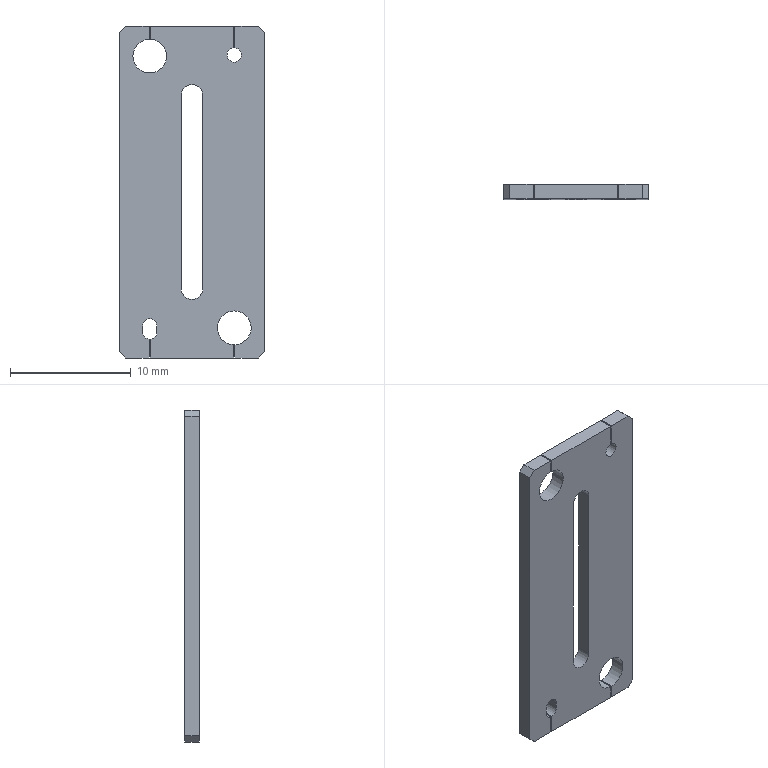Part | SolidWorks | features ICE 3, HoleWzd 2, Chamfer 1, Extrusion 1 | 1 solid | 37 faces | box 12 x 1.2 x 27.5 mm | volume 338.908 mm3 | plane 26 | cylinder 11 | commonest cylinder face diameters 1.2 x5 1.8 x3 2.8 x3
STEP:
#1=CARTESIAN_POINT('',(-3.5,-0.6,-10.5));
#2=VERTEX_POINT('',#1);
#3=CARTESIAN_POINT('',(-2.9,-0.6,-11.1));
#4=VERTEX_POINT('',#3);
#5=CARTESIAN_POINT('',(-3.5,-0.6,-11.1));
#6=DIRECTION('',(0.,1.,0.));
#7=DIRECTION('',(0.,0.,1.));
#8=AXIS2_PLACEMENT_3D('',#5,#6,#7);
#9=CIRCLE('',#8,0.6);
#10=EDGE_CURVE('',#2,#4,#9,.T.);
#11=ORIENTED_EDGE('',*,*,#10,.F.);
#12=CARTESIAN_POINT('',(-3.5,0.6,-10.5));
#13=VERTEX_POINT('',#12);
#14=CARTESIAN_POINT('',(-3.5,-0.6,-10.5));
#15=DIRECTION('',(0.,1.,0.));
#16=VECTOR('',#15,1000.);
#17=LINE('',#14,#16);
#18=EDGE_CURVE('',#2,#13,#17,.T.);
#19=ORIENTED_EDGE('',*,*,#18,.T.);
#20=CARTESIAN_POINT('',(-2.9,0.6,-11.1));
#21=VERTEX_POINT('',#20);
#22=CARTESIAN_POINT('',(-3.5,0.6,-11.1));
#23=DIRECTION('',(0.,1.,0.));
#24=DIRECTION('',(0.,0.,1.));
#25=AXIS2_PLACEMENT_3D('',#22,#23,#24);
#26=CIRCLE('',#25,0.6);
#27=EDGE_CURVE('',#13,#21,#26,.T.);
#28=ORIENTED_EDGE('',*,*,#27,.T.);
#29=CARTESIAN_POINT('',(-2.9,-0.6,-11.1));
#30=DIRECTION('',(0.,1.,0.));
#31=VECTOR('',#30,1000.);
#32=LINE('',#29,#31);
#33=EDGE_CURVE('',#4,#21,#32,.T.);
#34=ORIENTED_EDGE('',*,*,#33,.F.);
#35=EDGE_LOOP('',(#11,#19,#28,#34));
#36=FACE_OUTER_BOUND('',#35,.T.);
#37=CARTESIAN_POINT('',(-3.5,-0.6,-11.1));
#38=DIRECTION('',(0.,1.,0.));
#39=DIRECTION('',(0.,0.,1.));
#40=AXIS2_PLACEMENT_3D('',#37,#38,#39);
#41=CYLINDRICAL_SURFACE('',#40,0.6);
#42=ADVANCED_FACE('',(#36),#41,.F.);
#43=CARTESIAN_POINT('',(3.5,-0.6,-9.85));
#44=VERTEX_POINT('',#43);
#45=CARTESIAN_POINT('',(3.55,-0.6,-12.649));
#46=VERTEX_POINT('',#45);
#47=CARTESIAN_POINT('',(3.5,-0.6,-11.25));
#48=DIRECTION('',(0.,1.,0.));
#49=DIRECTION('',(0.,0.,1.));
#50=AXIS2_PLACEMENT_3D('',#47,#48,#49);
#51=CIRCLE('',#50,1.4);
#52=EDGE_CURVE('',#44,#46,#51,.T.);
#53=ORIENTED_EDGE('',*,*,#52,.F.);
#54=CARTESIAN_POINT('',(3.5,0.6,-9.85));
#55=VERTEX_POINT('',#54);
#56=CARTESIAN_POINT('',(3.5,0.6,-9.85));
#57=DIRECTION('',(0.,1.,0.));
#58=VECTOR('',#57,1000.);
#59=LINE('',#56,#58);
#60=EDGE_CURVE('',#44,#55,#59,.T.);
#61=ORIENTED_EDGE('',*,*,#60,.T.);
#62=CARTESIAN_POINT('',(3.55,0.6,-12.649));
#63=VERTEX_POINT('',#62);
#64=CARTESIAN_POINT('',(3.5,0.6,-11.25));
#65=DIRECTION('',(0.,1.,0.));
#66=DIRECTION('',(0.,0.,1.));
#67=AXIS2_PLACEMENT_3D('',#64,#65,#66);
#68=CIRCLE('',#67,1.4);
#69=EDGE_CURVE('',#55,#63,#68,.T.);
#70=ORIENTED_EDGE('',*,*,#69,.T.);
#71=CARTESIAN_POINT('',(3.55,0.6,-12.649));
#72=DIRECTION('',(0.,-1.,0.));
#73=VECTOR('',#72,1000.);
#74=LINE('',#71,#73);
#75=EDGE_CURVE('',#63,#46,#74,.T.);
#76=ORIENTED_EDGE('',*,*,#75,.T.);
#77=EDGE_LOOP('',(#53,#61,#70,#76));
#78=FACE_OUTER_BOUND('',#77,.T.);
#79=CARTESIAN_POINT('',(3.5,0.6,-11.25));
#80=DIRECTION('',(0.,1.,0.));
#81=DIRECTION('',(0.,0.,1.));
#82=AXIS2_PLACEMENT_3D('',#79,#80,#81);
#83=CYLINDRICAL_SURFACE('',#82,1.4);
#84=ADVANCED_FACE('',(#78),#83,.F.);
#85=CARTESIAN_POINT('',(0.,-0.6,8.9));
#86=VERTEX_POINT('',#85);
#87=CARTESIAN_POINT('',(0.9,-0.6,8.));
#88=VERTEX_POINT('',#87);
#89=CARTESIAN_POINT('',(0.,-0.6,8.));
#90=DIRECTION('',(0.,1.,0.));
#91=DIRECTION('',(0.,0.,1.));
#92=AXIS2_PLACEMENT_3D('',#89,#90,#91);
#93=CIRCLE('',#92,0.9);
#94=EDGE_CURVE('',#86,#88,#93,.T.);
#95=ORIENTED_EDGE('',*,*,#94,.F.);
#96=CARTESIAN_POINT('',(0.,0.6,8.9));
#97=VERTEX_POINT('',#96);
#98=CARTESIAN_POINT('',(0.,-0.6,8.9));
#99=DIRECTION('',(0.,1.,0.));
#100=VECTOR('',#99,1000.);
#101=LINE('',#98,#100);
#102=EDGE_CURVE('',#86,#97,#101,.T.);
#103=ORIENTED_EDGE('',*,*,#102,.T.);
#104=CARTESIAN_POINT('',(0.9,0.6,8.));
#105=VERTEX_POINT('',#104);
#106=CARTESIAN_POINT('',(0.,0.6,8.));
#107=DIRECTION('',(0.,1.,0.));
#108=DIRECTION('',(0.,0.,1.));
#109=AXIS2_PLACEMENT_3D('',#106,#107,#108);
#110=CIRCLE('',#109,0.9);
#111=EDGE_CURVE('',#97,#105,#110,.T.);
#112=ORIENTED_EDGE('',*,*,#111,.T.);
#113=CARTESIAN_POINT('',(0.9,-0.6,8.));
#114=DIRECTION('',(0.,1.,0.));
#115=VECTOR('',#114,1000.);
#116=LINE('',#113,#115);
#117=EDGE_CURVE('',#88,#105,#116,.T.);
#118=ORIENTED_EDGE('',*,*,#117,.F.);
#119=EDGE_LOOP('',(#95,#103,#112,#118));
#120=FACE_OUTER_BOUND('',#119,.T.);
#121=CARTESIAN_POINT('',(0.,-0.6,8.));
#122=DIRECTION('',(0.,1.,0.));
#123=DIRECTION('',(0.,0.,1.));
#124=AXIS2_PLACEMENT_3D('',#121,#122,#123);
#125=CYLINDRICAL_SURFACE('',#124,0.9);
#126=ADVANCED_FACE('',(#120),#125,.F.);
#127=CARTESIAN_POINT('',(3.45,-0.6,-13.75));
#128=VERTEX_POINT('',#127);
#129=CARTESIAN_POINT('',(-3.45,-0.6,-13.75));
#130=VERTEX_POINT('',#129);
#131=CARTESIAN_POINT('',(-6.,-0.6,-13.75));
#132=DIRECTION('',(-1.,0.,0.));
#133=VECTOR('',#132,1000.);
#134=LINE('',#131,#133);
#135=EDGE_CURVE('',#128,#130,#134,.T.);
#136=ORIENTED_EDGE('',*,*,#135,.T.);
#137=CARTESIAN_POINT('',(-3.45,0.6,-13.75));
#138=VERTEX_POINT('',#137);
#139=CARTESIAN_POINT('',(-3.45,-0.6,-13.75));
#140=DIRECTION('',(0.,1.,0.));
#141=VECTOR('',#140,1000.);
#142=LINE('',#139,#141);
#143=EDGE_CURVE('',#130,#138,#142,.T.);
#144=ORIENTED_EDGE('',*,*,#143,.T.);
#145=CARTESIAN_POINT('',(3.45,0.6,-13.75));
#146=VERTEX_POINT('',#145);
#147=CARTESIAN_POINT('',(-6.,0.6,-13.75));
#148=DIRECTION('',(-1.,0.,0.));
#149=VECTOR('',#148,1000.);
#150=LINE('',#147,#149);
#151=EDGE_CURVE('',#146,#138,#150,.T.);
#152=ORIENTED_EDGE('',*,*,#151,.F.);
#153=CARTESIAN_POINT('',(3.45,0.6,-13.75));
#154=DIRECTION('',(0.,-1.,0.));
#155=VECTOR('',#154,1000.);
#156=LINE('',#153,#155);
#157=EDGE_CURVE('',#146,#128,#156,.T.);
#158=ORIENTED_EDGE('',*,*,#157,.T.);
#159=EDGE_LOOP('',(#136,#144,#152,#158));
#160=FACE_OUTER_BOUND('',#159,.T.);
#161=CARTESIAN_POINT('',(-6.,0.6,-13.75));
#162=DIRECTION('',(0.,0.,1.));
#163=DIRECTION('',(1.,0.,0.));
#164=AXIS2_PLACEMENT_3D('',#161,#162,#163);
#165=PLANE('',#164);
#166=ADVANCED_FACE('',(#160),#165,.F.);
#167=CARTESIAN_POINT('',(-2.9,0.6,-11.6));
#168=VERTEX_POINT('',#167);
#169=CARTESIAN_POINT('',(-3.45,0.6,-12.198));
#170=VERTEX_POINT('',#169);
#171=CARTESIAN_POINT('',(-3.5,0.6,-11.6));
#172=DIRECTION('',(0.,1.,0.));
#173=DIRECTION('',(0.,0.,1.));
#174=AXIS2_PLACEMENT_3D('',#171,#172,#173);
#175=CIRCLE('',#174,0.6);
#176=EDGE_CURVE('',#168,#170,#175,.T.);
#177=ORIENTED_EDGE('',*,*,#176,.T.);
#178=CARTESIAN_POINT('',(-3.45,-0.6,-12.198));
#179=VERTEX_POINT('',#178);
#180=CARTESIAN_POINT('',(-3.45,-0.6,-12.198));
#181=DIRECTION('',(0.,-1.,0.));
#182=VECTOR('',#181,1000.);
#183=LINE('',#180,#182);
#184=EDGE_CURVE('',#170,#179,#183,.T.);
#185=ORIENTED_EDGE('',*,*,#184,.T.);
#186=CARTESIAN_POINT('',(-2.9,-0.6,-11.6));
#187=VERTEX_POINT('',#186);
#188=CARTESIAN_POINT('',(-3.5,-0.6,-11.6));
#189=DIRECTION('',(0.,1.,0.));
#190=DIRECTION('',(0.,0.,1.));
#191=AXIS2_PLACEMENT_3D('',#188,#189,#190);
#192=CIRCLE('',#191,0.6);
#193=EDGE_CURVE('',#187,#179,#192,.T.);
#194=ORIENTED_EDGE('',*,*,#193,.F.);
#195=CARTESIAN_POINT('',(-2.9,-0.6,-11.6));
#196=DIRECTION('',(0.,1.,0.));
#197=VECTOR('',#196,1000.);
#198=LINE('',#195,#197);
#199=EDGE_CURVE('',#187,#168,#198,.T.);
#200=ORIENTED_EDGE('',*,*,#199,.T.);
#201=EDGE_LOOP('',(#177,#185,#194,#200));
#202=FACE_OUTER_BOUND('',#201,.T.);
#203=CARTESIAN_POINT('',(-3.5,-0.6,-11.6));
#204=DIRECTION('',(0.,1.,0.));
#205=DIRECTION('',(0.,0.,1.));
#206=AXIS2_PLACEMENT_3D('',#203,#204,#205);
#207=CYLINDRICAL_SURFACE('',#206,0.6);
#208=ADVANCED_FACE('',(#202),#207,.F.);
#209=CARTESIAN_POINT('',(-3.45,0.6,13.75));
#210=VERTEX_POINT('',#209);
#211=CARTESIAN_POINT('',(3.45,0.6,13.75));
#212=VERTEX_POINT('',#211);
#213=CARTESIAN_POINT('',(-6.,0.6,13.75));
#214=DIRECTION('',(1.,0.,0.));
#215=VECTOR('',#214,1000.);
#216=LINE('',#213,#215);
#217=EDGE_CURVE('',#210,#212,#216,.T.);
#218=ORIENTED_EDGE('',*,*,#217,.F.);
#219=CARTESIAN_POINT('',(-3.45,-0.6,13.75));
#220=VERTEX_POINT('',#219);
#221=CARTESIAN_POINT('',(-3.45,-0.6,13.75));
#222=DIRECTION('',(0.,1.,0.));
#223=VECTOR('',#222,1000.);
#224=LINE('',#221,#223);
#225=EDGE_CURVE('',#220,#210,#224,.T.);
#226=ORIENTED_EDGE('',*,*,#225,.F.);
#227=CARTESIAN_POINT('',(3.45,-0.6,13.75));
#228=VERTEX_POINT('',#227);
#229=CARTESIAN_POINT('',(-6.,-0.6,13.75));
#230=DIRECTION('',(1.,0.,0.));
#231=VECTOR('',#230,1000.);
#232=LINE('',#229,#231);
#233=EDGE_CURVE('',#220,#228,#232,.T.);
#234=ORIENTED_EDGE('',*,*,#233,.T.);
#235=CARTESIAN_POINT('',(3.45,-0.6,13.75));
#236=DIRECTION('',(0.,1.,0.));
#237=VECTOR('',#236,1000.);
#238=LINE('',#235,#237);
#239=EDGE_CURVE('',#228,#212,#238,.T.);
#240=ORIENTED_EDGE('',*,*,#239,.T.);
#241=EDGE_LOOP('',(#218,#226,#234,#240));
#242=FACE_OUTER_BOUND('',#241,.T.);
#243=CARTESIAN_POINT('',(-6.,0.6,13.75));
#244=DIRECTION('',(0.,0.,-1.));
#245=DIRECTION('',(-1.,0.,0.));
#246=AXIS2_PLACEMENT_3D('',#243,#244,#245);
#247=PLANE('',#246);
#248=ADVANCED_FACE('',(#242),#247,.F.);
#249=CARTESIAN_POINT('',(3.55,0.6,13.75));
#250=VERTEX_POINT('',#249);
#251=CARTESIAN_POINT('',(5.5,0.6,13.75));
#252=VERTEX_POINT('',#251);
#253=CARTESIAN_POINT('',(-6.,0.6,13.75));
#254=DIRECTION('',(1.,0.,0.));
#255=VECTOR('',#254,1000.);
#256=LINE('',#253,#255);
#257=EDGE_CURVE('',#250,#252,#256,.T.);
#258=ORIENTED_EDGE('',*,*,#257,.F.);
#259=CARTESIAN_POINT('',(3.55,-0.6,13.75));
#260=VERTEX_POINT('',#259);
#261=CARTESIAN_POINT('',(3.55,-0.6,13.75));
#262=DIRECTION('',(0.,1.,0.));
#263=VECTOR('',#262,1000.);
#264=LINE('',#261,#263);
#265=EDGE_CURVE('',#260,#250,#264,.T.);
#266=ORIENTED_EDGE('',*,*,#265,.F.);
#267=CARTESIAN_POINT('',(5.5,-0.6,13.75));
#268=VERTEX_POINT('',#267);
#269=CARTESIAN_POINT('',(-6.,-0.6,13.75));
#270=DIRECTION('',(1.,0.,0.));
#271=VECTOR('',#270,1000.);
#272=LINE('',#269,#271);
#273=EDGE_CURVE('',#260,#268,#272,.T.);
#274=ORIENTED_EDGE('',*,*,#273,.T.);
#275=CARTESIAN_POINT('',(5.5,0.6,13.75));
#276=DIRECTION('',(0.,1.,0.));
#277=VECTOR('',#276,1000.);
#278=LINE('',#275,#277);
#279=EDGE_CURVE('',#268,#252,#278,.T.);
#280=ORIENTED_EDGE('',*,*,#279,.T.);
#281=EDGE_LOOP('',(#258,#266,#274,#280));
#282=FACE_OUTER_BOUND('',#281,.T.);
#283=CARTESIAN_POINT('',(-6.,0.6,13.75));
#284=DIRECTION('',(0.,0.,-1.));
#285=DIRECTION('',(-1.,0.,0.));
#286=AXIS2_PLACEMENT_3D('',#283,#284,#285);
#287=PLANE('',#286);
#288=ADVANCED_FACE('',(#282),#287,.F.);
#289=CARTESIAN_POINT('',(5.5,-0.6,-13.75));
#290=VERTEX_POINT('',#289);
#291=CARTESIAN_POINT('',(3.55,-0.6,-13.75));
#292=VERTEX_POINT('',#291);
#293=CARTESIAN_POINT('',(-6.,-0.6,-13.75));
#294=DIRECTION('',(-1.,0.,0.));
#295=VECTOR('',#294,1000.);
#296=LINE('',#293,#295);
#297=EDGE_CURVE('',#290,#292,#296,.T.);
#298=ORIENTED_EDGE('',*,*,#297,.T.);
#299=CARTESIAN_POINT('',(3.55,0.6,-13.75));
#300=VERTEX_POINT('',#299);
#301=CARTESIAN_POINT('',(3.55,0.6,-13.75));
#302=DIRECTION('',(0.,1.,0.));
#303=VECTOR('',#302,1000.);
#304=LINE('',#301,#303);
#305=EDGE_CURVE('',#292,#300,#304,.T.);
#306=ORIENTED_EDGE('',*,*,#305,.T.);
#307=CARTESIAN_POINT('',(5.5,0.6,-13.75));
#308=VERTEX_POINT('',#307);
#309=CARTESIAN_POINT('',(-6.,0.6,-13.75));
#310=DIRECTION('',(-1.,0.,0.));
#311=VECTOR('',#310,1000.);
#312=LINE('',#309,#311);
#313=EDGE_CURVE('',#308,#300,#312,.T.);
#314=ORIENTED_EDGE('',*,*,#313,.F.);
#315=CARTESIAN_POINT('',(5.5,0.6,-13.75));
#316=DIRECTION('',(0.,-1.,0.));
#317=VECTOR('',#316,1000.);
#318=LINE('',#315,#317);
#319=EDGE_CURVE('',#308,#290,#318,.T.);
#320=ORIENTED_EDGE('',*,*,#319,.T.);
#321=EDGE_LOOP('',(#298,#306,#314,#320));
#322=FACE_OUTER_BOUND('',#321,.T.);
#323=CARTESIAN_POINT('',(-6.,0.6,-13.75));
#324=DIRECTION('',(0.,0.,1.));
#325=DIRECTION('',(1.,0.,0.));
#326=AXIS2_PLACEMENT_3D('',#323,#324,#325);
#327=PLANE('',#326);
#328=ADVANCED_FACE('',(#322),#327,.F.);
#329=CARTESIAN_POINT('',(6.,-0.6,13.25));
#330=VERTEX_POINT('',#329);
#331=CARTESIAN_POINT('',(6.,-0.6,-13.25));
#332=VERTEX_POINT('',#331);
#333=CARTESIAN_POINT('',(6.,-0.6,-13.75));
#334=DIRECTION('',(0.,0.,-1.));
#335=VECTOR('',#334,1000.);
#336=LINE('',#333,#335);
#337=EDGE_CURVE('',#330,#332,#336,.T.);
#338=ORIENTED_EDGE('',*,*,#337,.T.);
#339=CARTESIAN_POINT('',(6.,0.6,-13.25));
#340=VERTEX_POINT('',#339);
#341=CARTESIAN_POINT('',(6.,0.6,-13.25));
#342=DIRECTION('',(0.,1.,0.));
#343=VECTOR('',#342,1000.);
#344=LINE('',#341,#343);
#345=EDGE_CURVE('',#332,#340,#344,.T.);
#346=ORIENTED_EDGE('',*,*,#345,.T.);
#347=CARTESIAN_POINT('',(6.,0.6,13.25));
#348=VERTEX_POINT('',#347);
#349=CARTESIAN_POINT('',(6.,0.6,-13.75));
#350=DIRECTION('',(0.,0.,-1.));
#351=VECTOR('',#350,1000.);
#352=LINE('',#349,#351);
#353=EDGE_CURVE('',#348,#340,#352,.T.);
#354=ORIENTED_EDGE('',*,*,#353,.F.);
#355=CARTESIAN_POINT('',(6.,0.6,13.25));
#356=DIRECTION('',(0.,-1.,0.));
#357=VECTOR('',#356,1000.);
#358=LINE('',#355,#357);
#359=EDGE_CURVE('',#348,#330,#358,.T.);
#360=ORIENTED_EDGE('',*,*,#359,.T.);
#361=EDGE_LOOP('',(#338,#346,#354,#360));
#362=FACE_OUTER_BOUND('',#361,.T.);
#363=CARTESIAN_POINT('',(6.,0.6,-13.75));
#364=DIRECTION('',(-1.,0.,0.));
#365=DIRECTION('',(0.,0.,1.));
#366=AXIS2_PLACEMENT_3D('',#363,#364,#365);
#367=PLANE('',#366);
#368=ADVANCED_FACE('',(#362),#367,.F.);
#369=CARTESIAN_POINT('',(-3.55,0.6,-13.75));
#370=VERTEX_POINT('',#369);
#371=CARTESIAN_POINT('',(-5.5,0.6,-13.75));
#372=VERTEX_POINT('',#371);
#373=CARTESIAN_POINT('',(-6.,0.6,-13.75));
#374=DIRECTION('',(-1.,0.,0.));
#375=VECTOR('',#374,1000.);
#376=LINE('',#373,#375);
#377=EDGE_CURVE('',#370,#372,#376,.T.);
#378=ORIENTED_EDGE('',*,*,#377,.F.);
#379=CARTESIAN_POINT('',(-3.55,-0.6,-13.75));
#380=VERTEX_POINT('',#379);
#381=CARTESIAN_POINT('',(-3.55,-0.6,-13.75));
#382=DIRECTION('',(0.,1.,0.));
#383=VECTOR('',#382,1000.);
#384=LINE('',#381,#383);
#385=EDGE_CURVE('',#380,#370,#384,.T.);
#386=ORIENTED_EDGE('',*,*,#385,.F.);
#387=CARTESIAN_POINT('',(-5.5,-0.6,-13.75));
#388=VERTEX_POINT('',#387);
#389=CARTESIAN_POINT('',(-6.,-0.6,-13.75));
#390=DIRECTION('',(-1.,0.,0.));
#391=VECTOR('',#390,1000.);
#392=LINE('',#389,#391);
#393=EDGE_CURVE('',#380,#388,#392,.T.);
#394=ORIENTED_EDGE('',*,*,#393,.T.);
#395=CARTESIAN_POINT('',(-5.5,0.6,-13.75));
#396=DIRECTION('',(0.,1.,0.));
#397=VECTOR('',#396,1000.);
#398=LINE('',#395,#397);
#399=EDGE_CURVE('',#388,#372,#398,.T.);
#400=ORIENTED_EDGE('',*,*,#399,.T.);
#401=EDGE_LOOP('',(#378,#386,#394,#400));
#402=FACE_OUTER_BOUND('',#401,.T.);
#403=CARTESIAN_POINT('',(-6.,0.6,-13.75));
#404=DIRECTION('',(0.,0.,1.));
#405=DIRECTION('',(1.,0.,0.));
#406=AXIS2_PLACEMENT_3D('',#403,#404,#405);
#407=PLANE('',#406);
#408=ADVANCED_FACE('',(#402),#407,.F.);
#409=CARTESIAN_POINT('',(-6.,0.6,-13.25));
#410=VERTEX_POINT('',#409);
#411=CARTESIAN_POINT('',(-6.,0.6,13.25));
#412=VERTEX_POINT('',#411);
#413=CARTESIAN_POINT('',(-6.,0.6,-13.75));
#414=DIRECTION('',(0.,0.,1.));
#415=VECTOR('',#414,1000.);
#416=LINE('',#413,#415);
#417=EDGE_CURVE('',#410,#412,#416,.T.);
#418=ORIENTED_EDGE('',*,*,#417,.F.);
#419=CARTESIAN_POINT('',(-6.,-0.6,-13.25));
#420=VERTEX_POINT('',#419);
#421=CARTESIAN_POINT('',(-6.,0.6,-13.25));
#422=DIRECTION('',(0.,-1.,0.));
#423=VECTOR('',#422,1000.);
#424=LINE('',#421,#423);
#425=EDGE_CURVE('',#410,#420,#424,.T.);
#426=ORIENTED_EDGE('',*,*,#425,.T.);
#427=CARTESIAN_POINT('',(-6.,-0.6,13.25));
#428=VERTEX_POINT('',#427);
#429=CARTESIAN_POINT('',(-6.,-0.6,-13.75));
#430=DIRECTION('',(0.,0.,1.));
#431=VECTOR('',#430,1000.);
#432=LINE('',#429,#431);
#433=EDGE_CURVE('',#420,#428,#432,.T.);
#434=ORIENTED_EDGE('',*,*,#433,.T.);
#435=CARTESIAN_POINT('',(-6.,0.6,13.25));
#436=DIRECTION('',(0.,1.,0.));
#437=VECTOR('',#436,1000.);
#438=LINE('',#435,#437);
#439=EDGE_CURVE('',#428,#412,#438,.T.);
#440=ORIENTED_EDGE('',*,*,#439,.T.);
#441=EDGE_LOOP('',(#418,#426,#434,#440));
#442=FACE_OUTER_BOUND('',#441,.T.);
#443=CARTESIAN_POINT('',(-6.,0.6,-13.75));
#444=DIRECTION('',(1.,0.,0.));
#445=DIRECTION('',(0.,0.,-1.));
#446=AXIS2_PLACEMENT_3D('',#443,#444,#445);
#447=PLANE('',#446);
#448=ADVANCED_FACE('',(#442),#447,.F.);
#449=CARTESIAN_POINT('',(-5.5,-0.6,13.75));
#450=VERTEX_POINT('',#449);
#451=CARTESIAN_POINT('',(-3.55,-0.6,13.75));
#452=VERTEX_POINT('',#451);
#453=CARTESIAN_POINT('',(-6.,-0.6,13.75));
#454=DIRECTION('',(1.,0.,0.));
#455=VECTOR('',#454,1000.);
#456=LINE('',#453,#455);
#457=EDGE_CURVE('',#450,#452,#456,.T.);
#458=ORIENTED_EDGE('',*,*,#457,.T.);
#459=CARTESIAN_POINT('',(-3.55,0.6,13.75));
#460=VERTEX_POINT('',#459);
#461=CARTESIAN_POINT('',(-3.55,-0.6,13.75));
#462=DIRECTION('',(0.,1.,0.));
#463=VECTOR('',#462,1000.);
#464=LINE('',#461,#463);
#465=EDGE_CURVE('',#452,#460,#464,.T.);
#466=ORIENTED_EDGE('',*,*,#465,.T.);
#467=CARTESIAN_POINT('',(-5.5,0.6,13.75));
#468=VERTEX_POINT('',#467);
#469=CARTESIAN_POINT('',(-6.,0.6,13.75));
#470=DIRECTION('',(1.,0.,0.));
#471=VECTOR('',#470,1000.);
#472=LINE('',#469,#471);
#473=EDGE_CURVE('',#468,#460,#472,.T.);
#474=ORIENTED_EDGE('',*,*,#473,.F.);
#475=CARTESIAN_POINT('',(-5.5,0.6,13.75));
#476=DIRECTION('',(0.,-1.,0.));
#477=VECTOR('',#476,1000.);
#478=LINE('',#475,#477);
#479=EDGE_CURVE('',#468,#450,#478,.T.);
#480=ORIENTED_EDGE('',*,*,#479,.T.);
#481=EDGE_LOOP('',(#458,#466,#474,#480));
#482=FACE_OUTER_BOUND('',#481,.T.);
#483=CARTESIAN_POINT('',(-6.,0.6,13.75));
#484=DIRECTION('',(0.,0.,-1.));
#485=DIRECTION('',(-1.,0.,0.));
#486=AXIS2_PLACEMENT_3D('',#483,#484,#485);
#487=PLANE('',#486);
#488=ADVANCED_FACE('',(#482),#487,.F.);
#489=CARTESIAN_POINT('',(-3.45,0.6,-11.75));
#490=DIRECTION('',(0.,0.,-1.));
#491=VECTOR('',#490,1000.);
#492=LINE('',#489,#491);
#493=EDGE_CURVE('',#170,#138,#492,.T.);
#494=ORIENTED_EDGE('',*,*,#493,.F.);
#495=ORIENTED_EDGE('',*,*,#176,.F.);
#496=CARTESIAN_POINT('',(-2.9,0.6,-11.6));
#497=DIRECTION('',(0.,0.,-1.));
#498=VECTOR('',#497,1000.);
#499=LINE('',#496,#498);
#500=EDGE_CURVE('',#21,#168,#499,.T.);
#501=ORIENTED_EDGE('',*,*,#500,.F.);
#502=ORIENTED_EDGE('',*,*,#27,.F.);
#503=CARTESIAN_POINT('',(-4.1,0.6,-11.1));
#504=VERTEX_POINT('',#503);
#505=CARTESIAN_POINT('',(-3.5,0.6,-11.1));
#506=DIRECTION('',(0.,1.,0.));
#507=DIRECTION('',(0.,0.,1.));
#508=AXIS2_PLACEMENT_3D('',#505,#506,#507);
#509=CIRCLE('',#508,0.6);
#510=EDGE_CURVE('',#504,#13,#509,.T.);
#511=ORIENTED_EDGE('',*,*,#510,.F.);
#512=CARTESIAN_POINT('',(-4.1,0.6,-11.6));
#513=VERTEX_POINT('',#512);
#514=CARTESIAN_POINT('',(-4.1,0.6,-11.6));
#515=DIRECTION('',(0.,0.,1.));
#516=VECTOR('',#515,1000.);
#517=LINE('',#514,#516);
#518=EDGE_CURVE('',#513,#504,#517,.T.);
#519=ORIENTED_EDGE('',*,*,#518,.F.);
#520=CARTESIAN_POINT('',(-3.55,0.6,-12.198));
#521=VERTEX_POINT('',#520);
#522=CARTESIAN_POINT('',(-3.5,0.6,-11.6));
#523=DIRECTION('',(0.,1.,0.));
#524=DIRECTION('',(0.,0.,1.));
#525=AXIS2_PLACEMENT_3D('',#522,#523,#524);
#526=CIRCLE('',#525,0.6);
#527=EDGE_CURVE('',#521,#513,#526,.T.);
#528=ORIENTED_EDGE('',*,*,#527,.F.);
#529=CARTESIAN_POINT('',(-3.55,0.6,-11.75));
#530=DIRECTION('',(0.,0.,1.));
#531=VECTOR('',#530,1000.);
#532=LINE('',#529,#531);
#533=EDGE_CURVE('',#370,#521,#532,.T.);
#534=ORIENTED_EDGE('',*,*,#533,.F.);
#535=ORIENTED_EDGE('',*,*,#377,.T.);
#536=CARTESIAN_POINT('',(-9.625,0.6,-9.625));
#537=DIRECTION('',(-0.7071,0.,0.7071));
#538=VECTOR('',#537,1000.);
#539=LINE('',#536,#538);
#540=EDGE_CURVE('',#372,#410,#539,.T.);
#541=ORIENTED_EDGE('',*,*,#540,.T.);
#542=ORIENTED_EDGE('',*,*,#417,.T.);
#543=CARTESIAN_POINT('',(-9.625,0.6,9.625));
#544=DIRECTION('',(0.7071,0.,0.7071));
#545=VECTOR('',#544,1000.);
#546=LINE('',#543,#545);
#547=EDGE_CURVE('',#412,#468,#546,.T.);
#548=ORIENTED_EDGE('',*,*,#547,.T.);
#549=ORIENTED_EDGE('',*,*,#473,.T.);
#550=CARTESIAN_POINT('',(-3.55,0.6,12.649));
#551=VERTEX_POINT('',#550);
#552=CARTESIAN_POINT('',(-3.55,0.6,13.75));
#553=DIRECTION('',(0.,0.,1.));
#554=VECTOR('',#553,1000.);
#555=LINE('',#552,#554);
#556=EDGE_CURVE('',#551,#460,#555,.T.);
#557=ORIENTED_EDGE('',*,*,#556,.F.);
#558=CARTESIAN_POINT('',(-3.45,0.6,12.649));
#559=VERTEX_POINT('',#558);
#560=CARTESIAN_POINT('',(-3.5,0.6,11.25));
#561=DIRECTION('',(0.,1.,0.));
#562=DIRECTION('',(0.,0.,1.));
#563=AXIS2_PLACEMENT_3D('',#560,#561,#562);
#564=CIRCLE('',#563,1.4);
#565=EDGE_CURVE('',#559,#551,#564,.T.);
#566=ORIENTED_EDGE('',*,*,#565,.F.);
#567=CARTESIAN_POINT('',(-3.45,0.6,13.75));
#568=DIRECTION('',(0.,0.,-1.));
#569=VECTOR('',#568,1000.);
#570=LINE('',#567,#569);
#571=EDGE_CURVE('',#210,#559,#570,.T.);
#572=ORIENTED_EDGE('',*,*,#571,.F.);
#573=ORIENTED_EDGE('',*,*,#217,.T.);
#574=CARTESIAN_POINT('',(3.45,0.6,11.948));
#575=VERTEX_POINT('',#574);
#576=CARTESIAN_POINT('',(3.45,0.6,11.75));
#577=DIRECTION('',(0.,0.,1.));
#578=VECTOR('',#577,1000.);
#579=LINE('',#576,#578);
#580=EDGE_CURVE('',#575,#212,#579,.T.);
#581=ORIENTED_EDGE('',*,*,#580,.F.);
#582=CARTESIAN_POINT('',(3.55,0.6,11.948));
#583=VERTEX_POINT('',#582);
#584=CARTESIAN_POINT('',(3.5,0.6,11.35));
#585=DIRECTION('',(0.,1.,0.));
#586=DIRECTION('',(0.,0.,1.));
#587=AXIS2_PLACEMENT_3D('',#584,#585,#586);
#588=CIRCLE('',#587,0.6);
#589=EDGE_CURVE('',#583,#575,#588,.T.);
#590=ORIENTED_EDGE('',*,*,#589,.F.);
#591=CARTESIAN_POINT('',(3.55,0.6,11.75));
#592=DIRECTION('',(0.,0.,-1.));
#593=VECTOR('',#592,1000.);
#594=LINE('',#591,#593);
#595=EDGE_CURVE('',#250,#583,#594,.T.);
#596=ORIENTED_EDGE('',*,*,#595,.F.);
#597=ORIENTED_EDGE('',*,*,#257,.T.);
#598=CARTESIAN_POINT('',(9.625,0.6,9.625));
#599=DIRECTION('',(0.7071,0.,-0.7071));
#600=VECTOR('',#599,1000.);
#601=LINE('',#598,#600);
#602=EDGE_CURVE('',#252,#348,#601,.T.);
#603=ORIENTED_EDGE('',*,*,#602,.T.);
#604=ORIENTED_EDGE('',*,*,#353,.T.);
#605=CARTESIAN_POINT('',(9.625,0.6,-9.625));
#606=DIRECTION('',(-0.7071,0.,-0.7071));
#607=VECTOR('',#606,1000.);
#608=LINE('',#605,#607);
#609=EDGE_CURVE('',#340,#308,#608,.T.);
#610=ORIENTED_EDGE('',*,*,#609,.T.);
#611=ORIENTED_EDGE('',*,*,#313,.T.);
#612=CARTESIAN_POINT('',(3.55,0.6,-14.15));
#613=DIRECTION('',(0.,0.,-1.));
#614=VECTOR('',#613,1000.);
#615=LINE('',#612,#614);
#616=EDGE_CURVE('',#63,#300,#615,.T.);
#617=ORIENTED_EDGE('',*,*,#616,.F.);
#618=ORIENTED_EDGE('',*,*,#69,.F.);
#619=CARTESIAN_POINT('',(3.45,0.6,-12.649));
#620=VERTEX_POINT('',#619);
#621=CARTESIAN_POINT('',(3.5,0.6,-11.25));
#622=DIRECTION('',(0.,1.,0.));
#623=DIRECTION('',(0.,0.,1.));
#624=AXIS2_PLACEMENT_3D('',#621,#622,#623);
#625=CIRCLE('',#624,1.4);
#626=EDGE_CURVE('',#620,#55,#625,.T.);
#627=ORIENTED_EDGE('',*,*,#626,.F.);
#628=CARTESIAN_POINT('',(3.45,0.6,-14.15));
#629=DIRECTION('',(0.,0.,1.));
#630=VECTOR('',#629,1000.);
#631=LINE('',#628,#630);
#632=EDGE_CURVE('',#146,#620,#631,.T.);
#633=ORIENTED_EDGE('',*,*,#632,.F.);
#634=ORIENTED_EDGE('',*,*,#151,.T.);
#635=EDGE_LOOP('',(#494,#495,#501,#502,#511,#519,#528,#534,#535,#541,#542,#548,#549,#557,#566,#572,#573,#581,#590,#596,#597,#603,#604,#610,#611,#617,#618,#627,#633,#634));
#636=FACE_OUTER_BOUND('',#635,.T.);
#637=CARTESIAN_POINT('',(0.9,0.6,-8.));
#638=VERTEX_POINT('',#637);
#639=CARTESIAN_POINT('',(-0.9,0.6,-8.));
#640=VERTEX_POINT('',#639);
#641=CARTESIAN_POINT('',(0.,0.6,-8.));
#642=DIRECTION('',(0.,1.,0.));
#643=DIRECTION('',(0.,0.,1.));
#644=AXIS2_PLACEMENT_3D('',#641,#642,#643);
#645=CIRCLE('',#644,0.9);
#646=EDGE_CURVE('',#638,#640,#645,.T.);
#647=ORIENTED_EDGE('',*,*,#646,.F.);
#648=CARTESIAN_POINT('',(0.9,0.6,-8.));
#649=DIRECTION('',(0.,0.,-1.));
#650=VECTOR('',#649,1000.);
#651=LINE('',#648,#650);
#652=EDGE_CURVE('',#105,#638,#651,.T.);
#653=ORIENTED_EDGE('',*,*,#652,.F.);
#654=ORIENTED_EDGE('',*,*,#111,.F.);
#655=CARTESIAN_POINT('',(-0.9,0.6,8.));
#656=VERTEX_POINT('',#655);
#657=CARTESIAN_POINT('',(0.,0.6,8.));
#658=DIRECTION('',(0.,1.,0.));
#659=DIRECTION('',(0.,0.,1.));
#660=AXIS2_PLACEMENT_3D('',#657,#658,#659);
#661=CIRCLE('',#660,0.9);
#662=EDGE_CURVE('',#656,#97,#661,.T.);
#663=ORIENTED_EDGE('',*,*,#662,.F.);
#664=CARTESIAN_POINT('',(-0.9,0.6,-8.));
#665=DIRECTION('',(0.,0.,1.));
#666=VECTOR('',#665,1000.);
#667=LINE('',#664,#666);
#668=EDGE_CURVE('',#640,#656,#667,.T.);
#669=ORIENTED_EDGE('',*,*,#668,.F.);
#670=EDGE_LOOP('',(#647,#653,#654,#663,#669));
#671=FACE_BOUND('',#670,.T.);
#672=CARTESIAN_POINT('',(0.,0.6,0.));
#673=DIRECTION('',(0.,1.,0.));
#674=DIRECTION('',(0.,0.,1.));
#675=AXIS2_PLACEMENT_3D('',#672,#673,#674);
#676=PLANE('',#675);
#677=ADVANCED_FACE('',(#636,#671),#676,.T.);
#678=ORIENTED_EDGE('',*,*,#193,.T.);
#679=CARTESIAN_POINT('',(-3.45,-0.6,-11.75));
#680=DIRECTION('',(0.,0.,-1.));
#681=VECTOR('',#680,1000.);
#682=LINE('',#679,#681);
#683=EDGE_CURVE('',#179,#130,#682,.T.);
#684=ORIENTED_EDGE('',*,*,#683,.T.);
#685=ORIENTED_EDGE('',*,*,#135,.F.);
#686=CARTESIAN_POINT('',(3.45,-0.6,-12.649));
#687=VERTEX_POINT('',#686);
#688=CARTESIAN_POINT('',(3.45,-0.6,-14.15));
#689=DIRECTION('',(0.,0.,1.));
#690=VECTOR('',#689,1000.);
#691=LINE('',#688,#690);
#692=EDGE_CURVE('',#128,#687,#691,.T.);
#693=ORIENTED_EDGE('',*,*,#692,.T.);
#694=CARTESIAN_POINT('',(3.5,-0.6,-11.25));
#695=DIRECTION('',(0.,1.,0.));
#696=DIRECTION('',(0.,0.,1.));
#697=AXIS2_PLACEMENT_3D('',#694,#695,#696);
#698=CIRCLE('',#697,1.4);
#699=EDGE_CURVE('',#687,#44,#698,.T.);
#700=ORIENTED_EDGE('',*,*,#699,.T.);
#701=ORIENTED_EDGE('',*,*,#52,.T.);
#702=CARTESIAN_POINT('',(3.55,-0.6,-14.15));
#703=DIRECTION('',(0.,0.,-1.));
#704=VECTOR('',#703,1000.);
#705=LINE('',#702,#704);
#706=EDGE_CURVE('',#46,#292,#705,.T.);
#707=ORIENTED_EDGE('',*,*,#706,.T.);
#708=ORIENTED_EDGE('',*,*,#297,.F.);
#709=CARTESIAN_POINT('',(5.5,-0.6,-13.75));
#710=DIRECTION('',(0.7071,0.,0.7071));
#711=VECTOR('',#710,1000.);
#712=LINE('',#709,#711);
#713=EDGE_CURVE('',#290,#332,#712,.T.);
#714=ORIENTED_EDGE('',*,*,#713,.T.);
#715=ORIENTED_EDGE('',*,*,#337,.F.);
#716=CARTESIAN_POINT('',(6.,-0.6,13.25));
#717=DIRECTION('',(-0.7071,0.,0.7071));
#718=VECTOR('',#717,1000.);
#719=LINE('',#716,#718);
#720=EDGE_CURVE('',#330,#268,#719,.T.);
#721=ORIENTED_EDGE('',*,*,#720,.T.);
#722=ORIENTED_EDGE('',*,*,#273,.F.);
#723=CARTESIAN_POINT('',(3.55,-0.6,11.948));
#724=VERTEX_POINT('',#723);
#725=CARTESIAN_POINT('',(3.55,-0.6,11.75));
#726=DIRECTION('',(0.,0.,-1.));
#727=VECTOR('',#726,1000.);
#728=LINE('',#725,#727);
#729=EDGE_CURVE('',#260,#724,#728,.T.);
#730=ORIENTED_EDGE('',*,*,#729,.T.);
#731=CARTESIAN_POINT('',(3.45,-0.6,11.948));
#732=VERTEX_POINT('',#731);
#733=CARTESIAN_POINT('',(3.5,-0.6,11.35));
#734=DIRECTION('',(0.,1.,0.));
#735=DIRECTION('',(0.,0.,1.));
#736=AXIS2_PLACEMENT_3D('',#733,#734,#735);
#737=CIRCLE('',#736,0.6);
#738=EDGE_CURVE('',#724,#732,#737,.T.);
#739=ORIENTED_EDGE('',*,*,#738,.T.);
#740=CARTESIAN_POINT('',(3.45,-0.6,11.75));
#741=DIRECTION('',(0.,0.,1.));
#742=VECTOR('',#741,1000.);
#743=LINE('',#740,#742);
#744=EDGE_CURVE('',#732,#228,#743,.T.);
#745=ORIENTED_EDGE('',*,*,#744,.T.);
#746=ORIENTED_EDGE('',*,*,#233,.F.);
#747=CARTESIAN_POINT('',(-3.45,-0.6,12.649));
#748=VERTEX_POINT('',#747);
#749=CARTESIAN_POINT('',(-3.45,-0.6,13.75));
#750=DIRECTION('',(0.,0.,-1.));
#751=VECTOR('',#750,1000.);
#752=LINE('',#749,#751);
#753=EDGE_CURVE('',#220,#748,#752,.T.);
#754=ORIENTED_EDGE('',*,*,#753,.T.);
#755=CARTESIAN_POINT('',(-3.55,-0.6,12.649));
#756=VERTEX_POINT('',#755);
#757=CARTESIAN_POINT('',(-3.5,-0.6,11.25));
#758=DIRECTION('',(0.,1.,0.));
#759=DIRECTION('',(0.,0.,1.));
#760=AXIS2_PLACEMENT_3D('',#757,#758,#759);
#761=CIRCLE('',#760,1.4);
#762=EDGE_CURVE('',#748,#756,#761,.T.);
#763=ORIENTED_EDGE('',*,*,#762,.T.);
#764=CARTESIAN_POINT('',(-3.55,-0.6,13.75));
#765=DIRECTION('',(0.,0.,1.));
#766=VECTOR('',#765,1000.);
#767=LINE('',#764,#766);
#768=EDGE_CURVE('',#756,#452,#767,.T.);
#769=ORIENTED_EDGE('',*,*,#768,.T.);
#770=ORIENTED_EDGE('',*,*,#457,.F.);
#771=CARTESIAN_POINT('',(-5.5,-0.6,13.75));
#772=DIRECTION('',(-0.7071,0.,-0.7071));
#773=VECTOR('',#772,1000.);
#774=LINE('',#771,#773);
#775=EDGE_CURVE('',#450,#428,#774,.T.);
#776=ORIENTED_EDGE('',*,*,#775,.T.);
#777=ORIENTED_EDGE('',*,*,#433,.F.);
#778=CARTESIAN_POINT('',(-6.,-0.6,-13.25));
#779=DIRECTION('',(0.7071,0.,-0.7071));
#780=VECTOR('',#779,1000.);
#781=LINE('',#778,#780);
#782=EDGE_CURVE('',#420,#388,#781,.T.);
#783=ORIENTED_EDGE('',*,*,#782,.T.);
#784=ORIENTED_EDGE('',*,*,#393,.F.);
#785=CARTESIAN_POINT('',(-3.55,-0.6,-12.198));
#786=VERTEX_POINT('',#785);
#787=CARTESIAN_POINT('',(-3.55,-0.6,-11.75));
#788=DIRECTION('',(0.,0.,1.));
#789=VECTOR('',#788,1000.);
#790=LINE('',#787,#789);
#791=EDGE_CURVE('',#380,#786,#790,.T.);
#792=ORIENTED_EDGE('',*,*,#791,.T.);
#793=CARTESIAN_POINT('',(-4.1,-0.6,-11.6));
#794=VERTEX_POINT('',#793);
#795=CARTESIAN_POINT('',(-3.5,-0.6,-11.6));
#796=DIRECTION('',(0.,1.,0.));
#797=DIRECTION('',(0.,0.,1.));
#798=AXIS2_PLACEMENT_3D('',#795,#796,#797);
#799=CIRCLE('',#798,0.6);
#800=EDGE_CURVE('',#786,#794,#799,.T.);
#801=ORIENTED_EDGE('',*,*,#800,.T.);
#802=CARTESIAN_POINT('',(-4.1,-0.6,-11.1));
#803=VERTEX_POINT('',#802);
#804=CARTESIAN_POINT('',(-4.1,-0.6,-11.6));
#805=DIRECTION('',(0.,0.,1.));
#806=VECTOR('',#805,1000.);
#807=LINE('',#804,#806);
#808=EDGE_CURVE('',#794,#803,#807,.T.);
#809=ORIENTED_EDGE('',*,*,#808,.T.);
#810=CARTESIAN_POINT('',(-3.5,-0.6,-11.1));
#811=DIRECTION('',(0.,1.,0.));
#812=DIRECTION('',(0.,0.,1.));
#813=AXIS2_PLACEMENT_3D('',#810,#811,#812);
#814=CIRCLE('',#813,0.6);
#815=EDGE_CURVE('',#803,#2,#814,.T.);
#816=ORIENTED_EDGE('',*,*,#815,.T.);
#817=ORIENTED_EDGE('',*,*,#10,.T.);
#818=CARTESIAN_POINT('',(-2.9,-0.6,-11.6));
#819=DIRECTION('',(0.,0.,-1.));
#820=VECTOR('',#819,1000.);
#821=LINE('',#818,#820);
#822=EDGE_CURVE('',#4,#187,#821,.T.);
#823=ORIENTED_EDGE('',*,*,#822,.T.);
#824=EDGE_LOOP('',(#678,#684,#685,#693,#700,#701,#707,#708,#714,#715,#721,#722,#730,#739,#745,#746,#754,#763,#769,#770,#776,#777,#783,#784,#792,#801,#809,#816,#817,#823));
#825=FACE_OUTER_BOUND('',#824,.T.);
#826=CARTESIAN_POINT('',(0.9,-0.6,-8.));
#827=VERTEX_POINT('',#826);
#828=CARTESIAN_POINT('',(0.9,-0.6,-8.));
#829=DIRECTION('',(0.,0.,-1.));
#830=VECTOR('',#829,1000.);
#831=LINE('',#828,#830);
#832=EDGE_CURVE('',#88,#827,#831,.T.);
#833=ORIENTED_EDGE('',*,*,#832,.T.);
#834=CARTESIAN_POINT('',(-0.9,-0.6,-8.));
#835=VERTEX_POINT('',#834);
#836=CARTESIAN_POINT('',(0.,-0.6,-8.));
#837=DIRECTION('',(0.,1.,0.));
#838=DIRECTION('',(0.,0.,1.));
#839=AXIS2_PLACEMENT_3D('',#836,#837,#838);
#840=CIRCLE('',#839,0.9);
#841=EDGE_CURVE('',#827,#835,#840,.T.);
#842=ORIENTED_EDGE('',*,*,#841,.T.);
#843=CARTESIAN_POINT('',(-0.9,-0.6,8.));
#844=VERTEX_POINT('',#843);
#845=CARTESIAN_POINT('',(-0.9,-0.6,-8.));
#846=DIRECTION('',(0.,0.,1.));
#847=VECTOR('',#846,1000.);
#848=LINE('',#845,#847);
#849=EDGE_CURVE('',#835,#844,#848,.T.);
#850=ORIENTED_EDGE('',*,*,#849,.T.);
#851=CARTESIAN_POINT('',(0.,-0.6,8.));
#852=DIRECTION('',(0.,1.,0.));
#853=DIRECTION('',(0.,0.,1.));
#854=AXIS2_PLACEMENT_3D('',#851,#852,#853);
#855=CIRCLE('',#854,0.9);
#856=EDGE_CURVE('',#844,#86,#855,.T.);
#857=ORIENTED_EDGE('',*,*,#856,.T.);
#858=ORIENTED_EDGE('',*,*,#94,.T.);
#859=EDGE_LOOP('',(#833,#842,#850,#857,#858));
#860=FACE_BOUND('',#859,.T.);
#861=CARTESIAN_POINT('',(0.,-0.6,0.));
#862=DIRECTION('',(0.,1.,0.));
#863=DIRECTION('',(0.,0.,1.));
#864=AXIS2_PLACEMENT_3D('',#861,#862,#863);
#865=PLANE('',#864);
#866=ADVANCED_FACE('',(#825,#860),#865,.F.);
#867=ORIENTED_EDGE('',*,*,#646,.T.);
#868=CARTESIAN_POINT('',(-0.9,-0.6,-8.));
#869=DIRECTION('',(0.,1.,0.));
#870=VECTOR('',#869,1000.);
#871=LINE('',#868,#870);
#872=EDGE_CURVE('',#835,#640,#871,.T.);
#873=ORIENTED_EDGE('',*,*,#872,.F.);
#874=ORIENTED_EDGE('',*,*,#841,.F.);
#875=CARTESIAN_POINT('',(0.9,-0.6,-8.));
#876=DIRECTION('',(0.,1.,0.));
#877=VECTOR('',#876,1000.);
#878=LINE('',#875,#877);
#879=EDGE_CURVE('',#827,#638,#878,.T.);
#880=ORIENTED_EDGE('',*,*,#879,.T.);
#881=EDGE_LOOP('',(#867,#873,#874,#880));
#882=FACE_OUTER_BOUND('',#881,.T.);
#883=CARTESIAN_POINT('',(0.,-0.6,-8.));
#884=DIRECTION('',(0.,1.,0.));
#885=DIRECTION('',(0.,0.,1.));
#886=AXIS2_PLACEMENT_3D('',#883,#884,#885);
#887=CYLINDRICAL_SURFACE('',#886,0.9);
#888=ADVANCED_FACE('',(#882),#887,.F.);
#889=ORIENTED_EDGE('',*,*,#652,.T.);
#890=ORIENTED_EDGE('',*,*,#879,.F.);
#891=ORIENTED_EDGE('',*,*,#832,.F.);
#892=ORIENTED_EDGE('',*,*,#117,.T.);
#893=EDGE_LOOP('',(#889,#890,#891,#892));
#894=FACE_OUTER_BOUND('',#893,.T.);
#895=CARTESIAN_POINT('',(0.9,-0.6,-8.));
#896=DIRECTION('',(1.,0.,0.));
#897=DIRECTION('',(0.,0.,-1.));
#898=AXIS2_PLACEMENT_3D('',#895,#896,#897);
#899=PLANE('',#898);
#900=ADVANCED_FACE('',(#894),#899,.F.);
#901=ORIENTED_EDGE('',*,*,#102,.F.);
#902=ORIENTED_EDGE('',*,*,#856,.F.);
#903=CARTESIAN_POINT('',(-0.9,-0.6,8.));
#904=DIRECTION('',(0.,1.,0.));
#905=VECTOR('',#904,1000.);
#906=LINE('',#903,#905);
#907=EDGE_CURVE('',#844,#656,#906,.T.);
#908=ORIENTED_EDGE('',*,*,#907,.T.);
#909=ORIENTED_EDGE('',*,*,#662,.T.);
#910=EDGE_LOOP('',(#901,#902,#908,#909));
#911=FACE_OUTER_BOUND('',#910,.T.);
#912=CARTESIAN_POINT('',(0.,-0.6,8.));
#913=DIRECTION('',(0.,1.,0.));
#914=DIRECTION('',(0.,0.,1.));
#915=AXIS2_PLACEMENT_3D('',#912,#913,#914);
#916=CYLINDRICAL_SURFACE('',#915,0.9);
#917=ADVANCED_FACE('',(#911),#916,.F.);
#918=ORIENTED_EDGE('',*,*,#668,.T.);
#919=ORIENTED_EDGE('',*,*,#907,.F.);
#920=ORIENTED_EDGE('',*,*,#849,.F.);
#921=ORIENTED_EDGE('',*,*,#872,.T.);
#922=EDGE_LOOP('',(#918,#919,#920,#921));
#923=FACE_OUTER_BOUND('',#922,.T.);
#924=CARTESIAN_POINT('',(-0.9,-0.6,-8.));
#925=DIRECTION('',(-1.,0.,0.));
#926=DIRECTION('',(0.,0.,1.));
#927=AXIS2_PLACEMENT_3D('',#924,#925,#926);
#928=PLANE('',#927);
#929=ADVANCED_FACE('',(#923),#928,.F.);
#930=ORIENTED_EDGE('',*,*,#540,.F.);
#931=ORIENTED_EDGE('',*,*,#399,.F.);
#932=ORIENTED_EDGE('',*,*,#782,.F.);
#933=ORIENTED_EDGE('',*,*,#425,.F.);
#934=EDGE_LOOP('',(#930,#931,#932,#933));
#935=FACE_OUTER_BOUND('',#934,.T.);
#936=CARTESIAN_POINT('',(-6.,0.6,-13.25));
#937=DIRECTION('',(0.7071,0.,0.7071));
#938=DIRECTION('',(0.,-1.,0.));
#939=AXIS2_PLACEMENT_3D('',#936,#937,#938);
#940=PLANE('',#939);
#941=ADVANCED_FACE('',(#935),#940,.F.);
#942=ORIENTED_EDGE('',*,*,#609,.F.);
#943=ORIENTED_EDGE('',*,*,#345,.F.);
#944=ORIENTED_EDGE('',*,*,#713,.F.);
#945=ORIENTED_EDGE('',*,*,#319,.F.);
#946=EDGE_LOOP('',(#942,#943,#944,#945));
#947=FACE_OUTER_BOUND('',#946,.T.);
#948=CARTESIAN_POINT('',(5.5,0.6,-13.75));
#949=DIRECTION('',(-0.7071,0.,0.7071));
#950=DIRECTION('',(0.,-1.,0.));
#951=AXIS2_PLACEMENT_3D('',#948,#949,#950);
#952=PLANE('',#951);
#953=ADVANCED_FACE('',(#947),#952,.F.);
#954=ORIENTED_EDGE('',*,*,#547,.F.);
#955=ORIENTED_EDGE('',*,*,#439,.F.);
#956=ORIENTED_EDGE('',*,*,#775,.F.);
#957=ORIENTED_EDGE('',*,*,#479,.F.);
#958=EDGE_LOOP('',(#954,#955,#956,#957));
#959=FACE_OUTER_BOUND('',#958,.T.);
#960=CARTESIAN_POINT('',(-5.5,0.6,13.75));
#961=DIRECTION('',(0.7071,0.,-0.7071));
#962=DIRECTION('',(0.,-1.,0.));
#963=AXIS2_PLACEMENT_3D('',#960,#961,#962);
#964=PLANE('',#963);
#965=ADVANCED_FACE('',(#959),#964,.F.);
#966=ORIENTED_EDGE('',*,*,#602,.F.);
#967=ORIENTED_EDGE('',*,*,#279,.F.);
#968=ORIENTED_EDGE('',*,*,#720,.F.);
#969=ORIENTED_EDGE('',*,*,#359,.F.);
#970=EDGE_LOOP('',(#966,#967,#968,#969));
#971=FACE_OUTER_BOUND('',#970,.T.);
#972=CARTESIAN_POINT('',(6.,0.6,13.25));
#973=DIRECTION('',(-0.7071,0.,-0.7071));
#974=DIRECTION('',(0.,-1.,0.));
#975=AXIS2_PLACEMENT_3D('',#972,#973,#974);
#976=PLANE('',#975);
#977=ADVANCED_FACE('',(#971),#976,.F.);
#978=ORIENTED_EDGE('',*,*,#738,.F.);
#979=CARTESIAN_POINT('',(3.55,0.6,11.948));
#980=DIRECTION('',(0.,1.,0.));
#981=VECTOR('',#980,1000.);
#982=LINE('',#979,#981);
#983=EDGE_CURVE('',#724,#583,#982,.T.);
#984=ORIENTED_EDGE('',*,*,#983,.T.);
#985=ORIENTED_EDGE('',*,*,#589,.T.);
#986=CARTESIAN_POINT('',(3.45,0.6,11.948));
#987=DIRECTION('',(0.,-1.,0.));
#988=VECTOR('',#987,1000.);
#989=LINE('',#986,#988);
#990=EDGE_CURVE('',#575,#732,#989,.T.);
#991=ORIENTED_EDGE('',*,*,#990,.T.);
#992=EDGE_LOOP('',(#978,#984,#985,#991));
#993=FACE_OUTER_BOUND('',#992,.T.);
#994=CARTESIAN_POINT('',(3.5,0.6,11.35));
#995=DIRECTION('',(0.,1.,0.));
#996=DIRECTION('',(0.,0.,1.));
#997=AXIS2_PLACEMENT_3D('',#994,#995,#996);
#998=CYLINDRICAL_SURFACE('',#997,0.6);
#999=ADVANCED_FACE('',(#993),#998,.F.);
#1000=ORIENTED_EDGE('',*,*,#762,.F.);
#1001=CARTESIAN_POINT('',(-3.45,0.6,12.649));
#1002=DIRECTION('',(0.,1.,0.));
#1003=VECTOR('',#1002,1000.);
#1004=LINE('',#1001,#1003);
#1005=EDGE_CURVE('',#748,#559,#1004,.T.);
#1006=ORIENTED_EDGE('',*,*,#1005,.T.);
#1007=ORIENTED_EDGE('',*,*,#565,.T.);
#1008=CARTESIAN_POINT('',(-3.55,0.6,12.649));
#1009=DIRECTION('',(0.,-1.,0.));
#1010=VECTOR('',#1009,1000.);
#1011=LINE('',#1008,#1010);
#1012=EDGE_CURVE('',#551,#756,#1011,.T.);
#1013=ORIENTED_EDGE('',*,*,#1012,.T.);
#1014=EDGE_LOOP('',(#1000,#1006,#1007,#1013));
#1015=FACE_OUTER_BOUND('',#1014,.T.);
#1016=CARTESIAN_POINT('',(-3.5,0.6,11.25));
#1017=DIRECTION('',(0.,1.,0.));
#1018=DIRECTION('',(0.,0.,1.));
#1019=AXIS2_PLACEMENT_3D('',#1016,#1017,#1018);
#1020=CYLINDRICAL_SURFACE('',#1019,1.4);
#1021=ADVANCED_FACE('',(#1015),#1020,.F.);
#1022=ORIENTED_EDGE('',*,*,#60,.F.);
#1023=ORIENTED_EDGE('',*,*,#699,.F.);
#1024=CARTESIAN_POINT('',(3.45,0.6,-12.649));
#1025=DIRECTION('',(0.,1.,0.));
#1026=VECTOR('',#1025,1000.);
#1027=LINE('',#1024,#1026);
#1028=EDGE_CURVE('',#687,#620,#1027,.T.);
#1029=ORIENTED_EDGE('',*,*,#1028,.T.);
#1030=ORIENTED_EDGE('',*,*,#626,.T.);
#1031=EDGE_LOOP('',(#1022,#1023,#1029,#1030));
#1032=FACE_OUTER_BOUND('',#1031,.T.);
#1033=CARTESIAN_POINT('',(3.5,0.6,-11.25));
#1034=DIRECTION('',(0.,1.,0.));
#1035=DIRECTION('',(0.,0.,1.));
#1036=AXIS2_PLACEMENT_3D('',#1033,#1034,#1035);
#1037=CYLINDRICAL_SURFACE('',#1036,1.4);
#1038=ADVANCED_FACE('',(#1032),#1037,.F.);
#1039=ORIENTED_EDGE('',*,*,#500,.T.);
#1040=ORIENTED_EDGE('',*,*,#199,.F.);
#1041=ORIENTED_EDGE('',*,*,#822,.F.);
#1042=ORIENTED_EDGE('',*,*,#33,.T.);
#1043=EDGE_LOOP('',(#1039,#1040,#1041,#1042));
#1044=FACE_OUTER_BOUND('',#1043,.T.);
#1045=CARTESIAN_POINT('',(-2.9,-0.6,-11.6));
#1046=DIRECTION('',(1.,0.,0.));
#1047=DIRECTION('',(0.,0.,-1.));
#1048=AXIS2_PLACEMENT_3D('',#1045,#1046,#1047);
#1049=PLANE('',#1048);
#1050=ADVANCED_FACE('',(#1044),#1049,.F.);
#1051=ORIENTED_EDGE('',*,*,#518,.T.);
#1052=CARTESIAN_POINT('',(-4.1,-0.6,-11.1));
#1053=DIRECTION('',(0.,1.,0.));
#1054=VECTOR('',#1053,1000.);
#1055=LINE('',#1052,#1054);
#1056=EDGE_CURVE('',#803,#504,#1055,.T.);
#1057=ORIENTED_EDGE('',*,*,#1056,.F.);
#1058=ORIENTED_EDGE('',*,*,#808,.F.);
#1059=CARTESIAN_POINT('',(-4.1,-0.6,-11.6));
#1060=DIRECTION('',(0.,1.,0.));
#1061=VECTOR('',#1060,1000.);
#1062=LINE('',#1059,#1061);
#1063=EDGE_CURVE('',#794,#513,#1062,.T.);
#1064=ORIENTED_EDGE('',*,*,#1063,.T.);
#1065=EDGE_LOOP('',(#1051,#1057,#1058,#1064));
#1066=FACE_OUTER_BOUND('',#1065,.T.);
#1067=CARTESIAN_POINT('',(-4.1,-0.6,-11.6));
#1068=DIRECTION('',(-1.,0.,0.));
#1069=DIRECTION('',(0.,0.,1.));
#1070=AXIS2_PLACEMENT_3D('',#1067,#1068,#1069);
#1071=PLANE('',#1070);
#1072=ADVANCED_FACE('',(#1066),#1071,.F.);
#1073=ORIENTED_EDGE('',*,*,#800,.F.);
#1074=CARTESIAN_POINT('',(-3.55,-0.6,-12.198));
#1075=DIRECTION('',(0.,1.,0.));
#1076=VECTOR('',#1075,1000.);
#1077=LINE('',#1074,#1076);
#1078=EDGE_CURVE('',#786,#521,#1077,.T.);
#1079=ORIENTED_EDGE('',*,*,#1078,.T.);
#1080=ORIENTED_EDGE('',*,*,#527,.T.);
#1081=ORIENTED_EDGE('',*,*,#1063,.F.);
#1082=EDGE_LOOP('',(#1073,#1079,#1080,#1081));
#1083=FACE_OUTER_BOUND('',#1082,.T.);
#1084=CARTESIAN_POINT('',(-3.5,-0.6,-11.6));
#1085=DIRECTION('',(0.,1.,0.));
#1086=DIRECTION('',(0.,0.,1.));
#1087=AXIS2_PLACEMENT_3D('',#1084,#1085,#1086);
#1088=CYLINDRICAL_SURFACE('',#1087,0.6);
#1089=ADVANCED_FACE('',(#1083),#1088,.F.);
#1090=ORIENTED_EDGE('',*,*,#18,.F.);
#1091=ORIENTED_EDGE('',*,*,#815,.F.);
#1092=ORIENTED_EDGE('',*,*,#1056,.T.);
#1093=ORIENTED_EDGE('',*,*,#510,.T.);
#1094=EDGE_LOOP('',(#1090,#1091,#1092,#1093));
#1095=FACE_OUTER_BOUND('',#1094,.T.);
#1096=CARTESIAN_POINT('',(-3.5,-0.6,-11.1));
#1097=DIRECTION('',(0.,1.,0.));
#1098=DIRECTION('',(0.,0.,1.));
#1099=AXIS2_PLACEMENT_3D('',#1096,#1097,#1098);
#1100=CYLINDRICAL_SURFACE('',#1099,0.6);
#1101=ADVANCED_FACE('',(#1095),#1100,.F.);
#1102=ORIENTED_EDGE('',*,*,#632,.T.);
#1103=ORIENTED_EDGE('',*,*,#1028,.F.);
#1104=ORIENTED_EDGE('',*,*,#692,.F.);
#1105=ORIENTED_EDGE('',*,*,#157,.F.);
#1106=EDGE_LOOP('',(#1102,#1103,#1104,#1105));
#1107=FACE_OUTER_BOUND('',#1106,.T.);
#1108=CARTESIAN_POINT('',(3.45,-0.6,-14.15));
#1109=DIRECTION('',(-1.,0.,0.));
#1110=DIRECTION('',(0.,0.,1.));
#1111=AXIS2_PLACEMENT_3D('',#1108,#1109,#1110);
#1112=PLANE('',#1111);
#1113=ADVANCED_FACE('',(#1107),#1112,.F.);
#1114=ORIENTED_EDGE('',*,*,#706,.F.);
#1115=ORIENTED_EDGE('',*,*,#75,.F.);
#1116=ORIENTED_EDGE('',*,*,#616,.T.);
#1117=ORIENTED_EDGE('',*,*,#305,.F.);
#1118=EDGE_LOOP('',(#1114,#1115,#1116,#1117));
#1119=FACE_OUTER_BOUND('',#1118,.T.);
#1120=CARTESIAN_POINT('',(3.55,-0.6,-14.15));
#1121=DIRECTION('',(1.,0.,0.));
#1122=DIRECTION('',(0.,0.,-1.));
#1123=AXIS2_PLACEMENT_3D('',#1120,#1121,#1122);
#1124=PLANE('',#1123);
#1125=ADVANCED_FACE('',(#1119),#1124,.F.);
#1126=ORIENTED_EDGE('',*,*,#580,.T.);
#1127=ORIENTED_EDGE('',*,*,#239,.F.);
#1128=ORIENTED_EDGE('',*,*,#744,.F.);
#1129=ORIENTED_EDGE('',*,*,#990,.F.);
#1130=EDGE_LOOP('',(#1126,#1127,#1128,#1129));
#1131=FACE_OUTER_BOUND('',#1130,.T.);
#1132=CARTESIAN_POINT('',(3.45,-0.6,11.75));
#1133=DIRECTION('',(-1.,0.,0.));
#1134=DIRECTION('',(0.,0.,1.));
#1135=AXIS2_PLACEMENT_3D('',#1132,#1133,#1134);
#1136=PLANE('',#1135);
#1137=ADVANCED_FACE('',(#1131),#1136,.F.);
#1138=ORIENTED_EDGE('',*,*,#729,.F.);
#1139=ORIENTED_EDGE('',*,*,#265,.T.);
#1140=ORIENTED_EDGE('',*,*,#595,.T.);
#1141=ORIENTED_EDGE('',*,*,#983,.F.);
#1142=EDGE_LOOP('',(#1138,#1139,#1140,#1141));
#1143=FACE_OUTER_BOUND('',#1142,.T.);
#1144=CARTESIAN_POINT('',(3.55,-0.6,11.75));
#1145=DIRECTION('',(1.,0.,0.));
#1146=DIRECTION('',(0.,0.,-1.));
#1147=AXIS2_PLACEMENT_3D('',#1144,#1145,#1146);
#1148=PLANE('',#1147);
#1149=ADVANCED_FACE('',(#1143),#1148,.F.);
#1150=ORIENTED_EDGE('',*,*,#556,.T.);
#1151=ORIENTED_EDGE('',*,*,#465,.F.);
#1152=ORIENTED_EDGE('',*,*,#768,.F.);
#1153=ORIENTED_EDGE('',*,*,#1012,.F.);
#1154=EDGE_LOOP('',(#1150,#1151,#1152,#1153));
#1155=FACE_OUTER_BOUND('',#1154,.T.);
#1156=CARTESIAN_POINT('',(-3.55,-0.6,13.75));
#1157=DIRECTION('',(-1.,0.,0.));
#1158=DIRECTION('',(0.,0.,1.));
#1159=AXIS2_PLACEMENT_3D('',#1156,#1157,#1158);
#1160=PLANE('',#1159);
#1161=ADVANCED_FACE('',(#1155),#1160,.F.);
#1162=ORIENTED_EDGE('',*,*,#753,.F.);
#1163=ORIENTED_EDGE('',*,*,#225,.T.);
#1164=ORIENTED_EDGE('',*,*,#571,.T.);
#1165=ORIENTED_EDGE('',*,*,#1005,.F.);
#1166=EDGE_LOOP('',(#1162,#1163,#1164,#1165));
#1167=FACE_OUTER_BOUND('',#1166,.T.);
#1168=CARTESIAN_POINT('',(-3.45,-0.6,13.75));
#1169=DIRECTION('',(1.,0.,0.));
#1170=DIRECTION('',(0.,0.,-1.));
#1171=AXIS2_PLACEMENT_3D('',#1168,#1169,#1170);
#1172=PLANE('',#1171);
#1173=ADVANCED_FACE('',(#1167),#1172,.F.);
#1174=ORIENTED_EDGE('',*,*,#791,.F.);
#1175=ORIENTED_EDGE('',*,*,#385,.T.);
#1176=ORIENTED_EDGE('',*,*,#533,.T.);
#1177=ORIENTED_EDGE('',*,*,#1078,.F.);
#1178=EDGE_LOOP('',(#1174,#1175,#1176,#1177));
#1179=FACE_OUTER_BOUND('',#1178,.T.);
#1180=CARTESIAN_POINT('',(-3.55,-0.6,-11.75));
#1181=DIRECTION('',(-1.,0.,0.));
#1182=DIRECTION('',(0.,0.,1.));
#1183=AXIS2_PLACEMENT_3D('',#1180,#1181,#1182);
#1184=PLANE('',#1183);
#1185=ADVANCED_FACE('',(#1179),#1184,.F.);
#1186=ORIENTED_EDGE('',*,*,#493,.T.);
#1187=ORIENTED_EDGE('',*,*,#143,.F.);
#1188=ORIENTED_EDGE('',*,*,#683,.F.);
#1189=ORIENTED_EDGE('',*,*,#184,.F.);
#1190=EDGE_LOOP('',(#1186,#1187,#1188,#1189));
#1191=FACE_OUTER_BOUND('',#1190,.T.);
#1192=CARTESIAN_POINT('',(-3.45,-0.6,-11.75));
#1193=DIRECTION('',(1.,0.,0.));
#1194=DIRECTION('',(0.,0.,-1.));
#1195=AXIS2_PLACEMENT_3D('',#1192,#1193,#1194);
#1196=PLANE('',#1195);
#1197=ADVANCED_FACE('',(#1191),#1196,.F.);
#1198=CLOSED_SHELL('',(#42,#84,#126,#166,#208,#248,#288,#328,#368,#408,#448,#488,#677,#866,#888,#900,#917,#929,#941,#953,#965,#977,#999,#1021,#1038,#1050,#1072,#1089,#1101,#1113,#1125,#1137,#1149,#1161,#1173,#1185,#1197));
#1199=MANIFOLD_SOLID_BREP('',#1198);
#1200=CARTESIAN_POINT('',(0.,0.,0.));
#1201=DIRECTION('',(0.,0.,1.));
#1202=DIRECTION('',(1.,0.,0.));
#1203=AXIS2_PLACEMENT_3D('',#1200,#1201,#1202);
#1204=(LENGTH_UNIT()NAMED_UNIT(*)SI_UNIT(.MILLI.,.METRE.));
#1205=UNCERTAINTY_MEASURE_WITH_UNIT(LENGTH_MEASURE(0.00001),#1204,'','');
#1206=(NAMED_UNIT(*)PLANE_ANGLE_UNIT()SI_UNIT($,.RADIAN.));
#1207=(NAMED_UNIT(*)SI_UNIT($,.STERADIAN.)SOLID_ANGLE_UNIT());
#1208=(GEOMETRIC_REPRESENTATION_CONTEXT(3)GLOBAL_UNCERTAINTY_ASSIGNED_CONTEXT((#1205))GLOBAL_UNIT_ASSIGNED_CONTEXT((#1204,#1206,#1207))REPRESENTATION_CONTEXT('',''));
#1209=ADVANCED_BREP_SHAPE_REPRESENTATION('',(#1199,#1203),#1208);